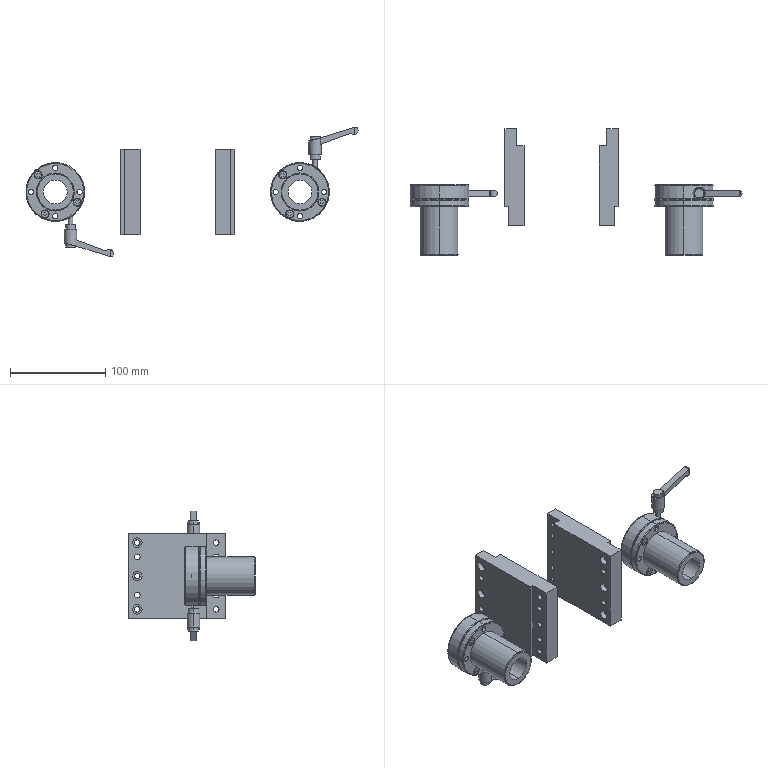Part | NX | features BREP 7 | 8 solids | 378 faces | box 349 x 133 x 136.523 mm | volume 512669 mm3 | cylinder 176 | plane 122 | torus 56 | cone 24 | commonest cylinder face diameters 5.5 x32 5.8 x24 10 x24 6 x16 9 x16 8.5 x12